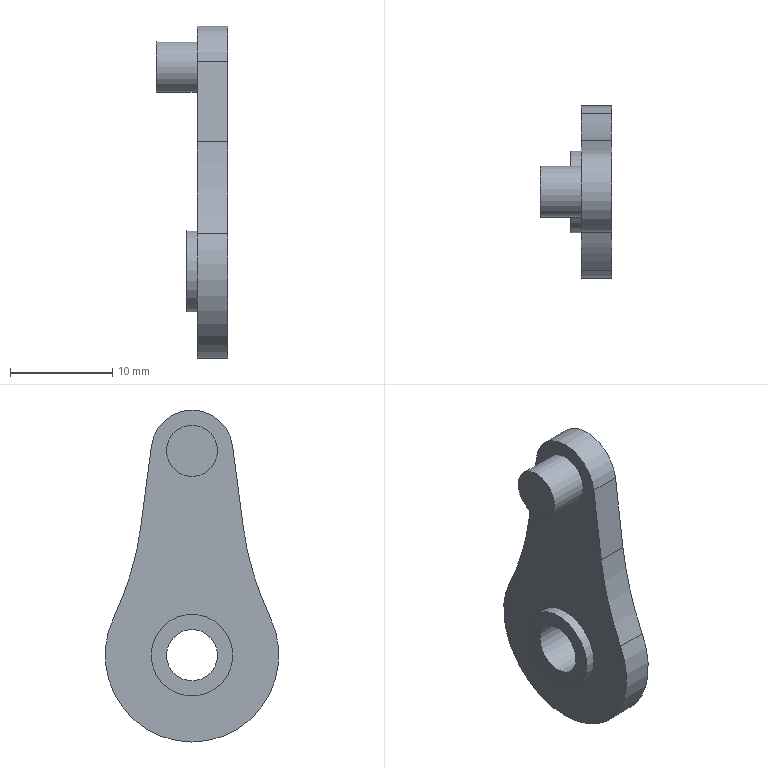Part | STEP file | COMPOUND | 2 solids | 15 faces | box 7 x 17 x 32.5 mm | volume 1174 mm3 | cylinder 8 | plane 7 | commonest cylinder face diameters 8 x3 5 x2 60 x2 17 x1
STEP:
#1=CARTESIAN_POINT('',(0.,0.,0.));
#2=DIRECTION('',(0.,0.,1.));
#3=DIRECTION('',(1.,0.,0.));
#4=AXIS2_PLACEMENT_3D('',#1,#2,#3);
#5=CARTESIAN_POINT('',(3.,4.,-20.));
#6=VERTEX_POINT('',#5);
#7=CARTESIAN_POINT('',(3.,0.,-20.));
#8=DIRECTION('',(1.,0.,0.));
#9=DIRECTION('',(0.,1.,0.));
#10=AXIS2_PLACEMENT_3D('',#7,#8,#9);
#11=CIRCLE('',#10,4.);
#12=CARTESIAN_POINT('',(3.,-1.072,-20.));
#13=DIRECTION('',(1.,0.,0.));
#14=DIRECTION('',(0.,1.,0.));
#15=AXIS2_PLACEMENT_3D('',#12,#13,#14);
#16=PLANE('',#15);
#17=CARTESIAN_POINT('',(1.072,0.));
#18=DIRECTION('',(1.,0.));
#19=AXIS2_PLACEMENT_2D('',#17,#18);
#20=CIRCLE('',#19,4.);
#21=(GEOMETRIC_REPRESENTATION_CONTEXT(2)PARAMETRIC_REPRESENTATION_CONTEXT()REPRESENTATION_CONTEXT('',''));
#22=DEFINITIONAL_REPRESENTATION('',(#20),#21);
#23=PCURVE('',#16,#22);
#24=CARTESIAN_POINT('',(3.,0.,-20.));
#25=DIRECTION('',(-1.,0.,0.));
#26=DIRECTION('',(0.,1.,0.));
#27=AXIS2_PLACEMENT_3D('',#24,#25,#26);
#28=CYLINDRICAL_SURFACE('',#27,4.);
#29=CARTESIAN_POINT('',(6.283,0.));
#30=DIRECTION('',(-1.,0.));
#31=VECTOR('',#30,1.);
#32=LINE('',#29,#31);
#33=(GEOMETRIC_REPRESENTATION_CONTEXT(2)PARAMETRIC_REPRESENTATION_CONTEXT()REPRESENTATION_CONTEXT('',''));
#34=DEFINITIONAL_REPRESENTATION('',(#32),#33);
#35=PCURVE('',#28,#34);
#36=SURFACE_CURVE('',#11,(#23,#35),.PCURVE_S1.);
#37=EDGE_CURVE('',#6,#6,#36,.T.);
#38=ORIENTED_EDGE('',*,*,#37,.T.);
#39=EDGE_LOOP('',(#38));
#40=FACE_BOUND('',#39,.T.);
#41=CARTESIAN_POINT('',(3.,2.5,-20.));
#42=VERTEX_POINT('',#41);
#43=CARTESIAN_POINT('',(3.,0.,-20.));
#44=DIRECTION('',(-1.,0.,0.));
#45=DIRECTION('',(0.,1.,0.));
#46=AXIS2_PLACEMENT_3D('',#43,#44,#45);
#47=CIRCLE('',#46,2.5);
#48=CARTESIAN_POINT('',(3.572,0.));
#49=CARTESIAN_POINT('',(3.572,-4.33));
#50=CARTESIAN_POINT('',(-0.1782,-2.165));
#51=CARTESIAN_POINT('',(-3.928,0.));
#52=CARTESIAN_POINT('',(-0.1782,2.165));
#53=CARTESIAN_POINT('',(3.572,4.33));
#54=CARTESIAN_POINT('',(3.572,0.));
#55=(BOUNDED_CURVE()B_SPLINE_CURVE(2,(#48,#49,#50,#51,#52,#53,#54),.UNSPECIFIED.,.T.,.F.)B_SPLINE_CURVE_WITH_KNOTS((1,2,2,2,2,1),(-2.094,0.,2.094,4.189,6.283,8.378),.UNSPECIFIED.)CURVE()GEOMETRIC_REPRESENTATION_ITEM()RATIONAL_B_SPLINE_CURVE((1.,0.5,1.,0.5,1.,0.5,1.))REPRESENTATION_ITEM(''));
#56=(GEOMETRIC_REPRESENTATION_CONTEXT(2)PARAMETRIC_REPRESENTATION_CONTEXT()REPRESENTATION_CONTEXT('',''));
#57=DEFINITIONAL_REPRESENTATION('',(#55),#56);
#58=PCURVE('',#16,#57);
#59=CARTESIAN_POINT('',(3.,0.,-20.));
#60=DIRECTION('',(-1.,0.,0.));
#61=DIRECTION('',(0.,1.,0.));
#62=AXIS2_PLACEMENT_3D('',#59,#60,#61);
#63=CYLINDRICAL_SURFACE('',#62,2.5);
#64=CARTESIAN_POINT('',(0.,0.));
#65=DIRECTION('',(1.,0.));
#66=VECTOR('',#65,1.);
#67=LINE('',#64,#66);
#68=(GEOMETRIC_REPRESENTATION_CONTEXT(2)PARAMETRIC_REPRESENTATION_CONTEXT()REPRESENTATION_CONTEXT('',''));
#69=DEFINITIONAL_REPRESENTATION('',(#67),#68);
#70=PCURVE('',#63,#69);
#71=SURFACE_CURVE('',#47,(#58,#70),.PCURVE_S1.);
#72=EDGE_CURVE('',#42,#42,#71,.T.);
#73=ORIENTED_EDGE('',*,*,#72,.T.);
#74=EDGE_LOOP('',(#73));
#75=FACE_BOUND('',#74,.T.);
#76=ADVANCED_FACE('',(#40,#75),#16,.T.);
#77=CARTESIAN_POINT('',(-1.,4.,-20.));
#78=VERTEX_POINT('',#77);
#79=CARTESIAN_POINT('',(-1.,0.,-20.));
#80=DIRECTION('',(1.,0.,0.));
#81=DIRECTION('',(0.,1.,0.));
#82=AXIS2_PLACEMENT_3D('',#79,#80,#81);
#83=CIRCLE('',#82,4.);
#84=CARTESIAN_POINT('',(-1.,-1.072,-20.));
#85=DIRECTION('',(1.,0.,0.));
#86=DIRECTION('',(0.,1.,0.));
#87=AXIS2_PLACEMENT_3D('',#84,#85,#86);
#88=PLANE('',#87);
#89=CARTESIAN_POINT('',(1.072,0.));
#90=DIRECTION('',(1.,0.));
#91=AXIS2_PLACEMENT_2D('',#89,#90);
#92=CIRCLE('',#91,4.);
#93=(GEOMETRIC_REPRESENTATION_CONTEXT(2)PARAMETRIC_REPRESENTATION_CONTEXT()REPRESENTATION_CONTEXT('',''));
#94=DEFINITIONAL_REPRESENTATION('',(#92),#93);
#95=PCURVE('',#88,#94);
#96=CARTESIAN_POINT('',(6.283,4.));
#97=DIRECTION('',(-1.,0.));
#98=VECTOR('',#97,1.);
#99=LINE('',#96,#98);
#100=(GEOMETRIC_REPRESENTATION_CONTEXT(2)PARAMETRIC_REPRESENTATION_CONTEXT()REPRESENTATION_CONTEXT('',''));
#101=DEFINITIONAL_REPRESENTATION('',(#99),#100);
#102=PCURVE('',#28,#101);
#103=SURFACE_CURVE('',#83,(#95,#102),.PCURVE_S1.);
#104=EDGE_CURVE('',#78,#78,#103,.T.);
#105=ORIENTED_EDGE('',*,*,#104,.T.);
#106=EDGE_LOOP('',(#105));
#107=FACE_BOUND('',#106,.F.);
#108=CARTESIAN_POINT('',(-1.,2.5,-20.));
#109=VERTEX_POINT('',#108);
#110=CARTESIAN_POINT('',(-1.,0.,-20.));
#111=DIRECTION('',(-1.,0.,0.));
#112=DIRECTION('',(0.,1.,0.));
#113=AXIS2_PLACEMENT_3D('',#110,#111,#112);
#114=CIRCLE('',#113,2.5);
#115=CARTESIAN_POINT('',(3.572,0.));
#116=CARTESIAN_POINT('',(3.572,-4.33));
#117=CARTESIAN_POINT('',(-0.1782,-2.165));
#118=CARTESIAN_POINT('',(-3.928,0.));
#119=CARTESIAN_POINT('',(-0.1782,2.165));
#120=CARTESIAN_POINT('',(3.572,4.33));
#121=CARTESIAN_POINT('',(3.572,0.));
#122=(BOUNDED_CURVE()B_SPLINE_CURVE(2,(#115,#116,#117,#118,#119,#120,#121),.UNSPECIFIED.,.T.,.F.)B_SPLINE_CURVE_WITH_KNOTS((1,2,2,2,2,1),(-2.094,0.,2.094,4.189,6.283,8.378),.UNSPECIFIED.)CURVE()GEOMETRIC_REPRESENTATION_ITEM()RATIONAL_B_SPLINE_CURVE((1.,0.5,1.,0.5,1.,0.5,1.))REPRESENTATION_ITEM(''));
#123=(GEOMETRIC_REPRESENTATION_CONTEXT(2)PARAMETRIC_REPRESENTATION_CONTEXT()REPRESENTATION_CONTEXT('',''));
#124=DEFINITIONAL_REPRESENTATION('',(#122),#123);
#125=PCURVE('',#88,#124);
#126=CARTESIAN_POINT('',(0.,4.));
#127=DIRECTION('',(1.,0.));
#128=VECTOR('',#127,1.);
#129=LINE('',#126,#128);
#130=(GEOMETRIC_REPRESENTATION_CONTEXT(2)PARAMETRIC_REPRESENTATION_CONTEXT()REPRESENTATION_CONTEXT('',''));
#131=DEFINITIONAL_REPRESENTATION('',(#129),#130);
#132=PCURVE('',#63,#131);
#133=SURFACE_CURVE('',#114,(#125,#132),.PCURVE_S1.);
#134=EDGE_CURVE('',#109,#109,#133,.T.);
#135=ORIENTED_EDGE('',*,*,#134,.T.);
#136=EDGE_LOOP('',(#135));
#137=FACE_BOUND('',#136,.F.);
#138=ADVANCED_FACE('',(#107,#137),#88,.F.);
#139=CARTESIAN_POINT('',(3.,4.,-20.));
#140=DIRECTION('',(-1.,0.,0.));
#141=VECTOR('',#140,1.);
#142=LINE('',#139,#141);
#143=CARTESIAN_POINT('',(6.283,0.));
#144=DIRECTION('',(0.,1.));
#145=VECTOR('',#144,1.);
#146=LINE('',#143,#145);
#147=(GEOMETRIC_REPRESENTATION_CONTEXT(2)PARAMETRIC_REPRESENTATION_CONTEXT()REPRESENTATION_CONTEXT('',''));
#148=DEFINITIONAL_REPRESENTATION('',(#146),#147);
#149=PCURVE('',#28,#148);
#150=CARTESIAN_POINT('',(0.,0.));
#151=DIRECTION('',(0.,1.));
#152=VECTOR('',#151,1.);
#153=LINE('',#150,#152);
#154=(GEOMETRIC_REPRESENTATION_CONTEXT(2)PARAMETRIC_REPRESENTATION_CONTEXT()REPRESENTATION_CONTEXT('',''));
#155=DEFINITIONAL_REPRESENTATION('',(#153),#154);
#156=PCURVE('',#28,#155);
#157=SEAM_CURVE('',#142,(#149,#156),.PCURVE_S1.);
#158=EDGE_CURVE('',#6,#78,#157,.T.);
#159=ORIENTED_EDGE('',*,*,#158,.T.);
#160=ORIENTED_EDGE('',*,*,#104,.T.);
#161=ORIENTED_EDGE('',*,*,#158,.F.);
#162=ORIENTED_EDGE('',*,*,#37,.F.);
#163=EDGE_LOOP('',(#159,#160,#161,#162));
#164=FACE_BOUND('',#163,.T.);
#165=ADVANCED_FACE('',(#164),#28,.T.);
#166=ORIENTED_EDGE('',*,*,#72,.T.);
#167=CARTESIAN_POINT('',(3.,2.5,-20.));
#168=DIRECTION('',(-1.,0.,0.));
#169=VECTOR('',#168,1.);
#170=LINE('',#167,#169);
#171=CARTESIAN_POINT('',(6.283,0.));
#172=DIRECTION('',(0.,1.));
#173=VECTOR('',#172,1.);
#174=LINE('',#171,#173);
#175=(GEOMETRIC_REPRESENTATION_CONTEXT(2)PARAMETRIC_REPRESENTATION_CONTEXT()REPRESENTATION_CONTEXT('',''));
#176=DEFINITIONAL_REPRESENTATION('',(#174),#175);
#177=PCURVE('',#63,#176);
#178=CARTESIAN_POINT('',(0.,0.));
#179=DIRECTION('',(0.,1.));
#180=VECTOR('',#179,1.);
#181=LINE('',#178,#180);
#182=(GEOMETRIC_REPRESENTATION_CONTEXT(2)PARAMETRIC_REPRESENTATION_CONTEXT()REPRESENTATION_CONTEXT('',''));
#183=DEFINITIONAL_REPRESENTATION('',(#181),#182);
#184=PCURVE('',#63,#183);
#185=SEAM_CURVE('',#170,(#177,#184),.PCURVE_S1.);
#186=EDGE_CURVE('',#42,#109,#185,.T.);
#187=ORIENTED_EDGE('',*,*,#186,.T.);
#188=ORIENTED_EDGE('',*,*,#134,.F.);
#189=ORIENTED_EDGE('',*,*,#186,.F.);
#190=EDGE_LOOP('',(#166,#187,#188,#189));
#191=FACE_BOUND('',#190,.F.);
#192=ADVANCED_FACE('',(#191),#63,.F.);
#193=CLOSED_SHELL('',(#76,#138,#165,#192));
#194=MANIFOLD_SOLID_BREP('',#193);
#195=CARTESIAN_POINT('',(3.,3.966,0.5224));
#196=VERTEX_POINT('',#195);
#197=CARTESIAN_POINT('',(3.,-3.966,0.5224));
#198=VERTEX_POINT('',#197);
#199=CARTESIAN_POINT('',(3.,0.,0.));
#200=DIRECTION('',(1.,0.,0.));
#201=DIRECTION('',(0.,0.9914,0.1306));
#202=AXIS2_PLACEMENT_3D('',#199,#200,#201);
#203=CIRCLE('',#202,4.);
#204=CARTESIAN_POINT('',(3.,2.773,-12.25));
#205=DIRECTION('',(1.,0.,0.));
#206=DIRECTION('',(0.,1.,0.));
#207=AXIS2_PLACEMENT_3D('',#204,#205,#206);
#208=PLANE('',#207);
#209=CARTESIAN_POINT('',(-2.773,12.25));
#210=DIRECTION('',(0.9914,0.1306));
#211=AXIS2_PLACEMENT_2D('',#209,#210);
#212=CIRCLE('',#211,4.);
#213=(GEOMETRIC_REPRESENTATION_CONTEXT(2)PARAMETRIC_REPRESENTATION_CONTEXT()REPRESENTATION_CONTEXT('',''));
#214=DEFINITIONAL_REPRESENTATION('',(#212),#213);
#215=PCURVE('',#208,#214);
#216=CARTESIAN_POINT('',(0.,0.,0.));
#217=DIRECTION('',(1.,0.,0.));
#218=DIRECTION('',(0.,0.9914,0.1306));
#219=AXIS2_PLACEMENT_3D('',#216,#217,#218);
#220=CYLINDRICAL_SURFACE('',#219,4.);
#221=CARTESIAN_POINT('',(0.,3.));
#222=DIRECTION('',(1.,0.));
#223=VECTOR('',#222,1.);
#224=LINE('',#221,#223);
#225=(GEOMETRIC_REPRESENTATION_CONTEXT(2)PARAMETRIC_REPRESENTATION_CONTEXT()REPRESENTATION_CONTEXT('',''));
#226=DEFINITIONAL_REPRESENTATION('',(#224),#225);
#227=PCURVE('',#220,#226);
#228=SURFACE_CURVE('',#203,(#215,#227),.PCURVE_S1.);
#229=EDGE_CURVE('',#196,#198,#228,.T.);
#230=ORIENTED_EDGE('',*,*,#229,.T.);
#231=CARTESIAN_POINT('',(3.,-5.,-7.33));
#232=VERTEX_POINT('',#231);
#233=CARTESIAN_POINT('',(3.,-3.966,0.5224));
#234=DIRECTION('',(0.,-0.1306,-0.9914));
#235=VECTOR('',#234,1.);
#236=LINE('',#233,#235);
#237=CARTESIAN_POINT('',(-6.738,12.772));
#238=DIRECTION('',(-0.1306,-0.9914));
#239=VECTOR('',#238,1.);
#240=LINE('',#237,#239);
#241=(GEOMETRIC_REPRESENTATION_CONTEXT(2)PARAMETRIC_REPRESENTATION_CONTEXT()REPRESENTATION_CONTEXT('',''));
#242=DEFINITIONAL_REPRESENTATION('',(#240),#241);
#243=PCURVE('',#208,#242);
#244=CARTESIAN_POINT('',(1.5,-4.483,-3.404));
#245=DIRECTION('',(0.,-0.9914,0.1306));
#246=DIRECTION('',(0.,-0.1306,-0.9914));
#247=AXIS2_PLACEMENT_3D('',#244,#245,#246);
#248=PLANE('',#247);
#249=CARTESIAN_POINT('',(-3.96,1.5));
#250=DIRECTION('',(1.,0.));
#251=VECTOR('',#250,1.);
#252=LINE('',#249,#251);
#253=(GEOMETRIC_REPRESENTATION_CONTEXT(2)PARAMETRIC_REPRESENTATION_CONTEXT()REPRESENTATION_CONTEXT('',''));
#254=DEFINITIONAL_REPRESENTATION('',(#252),#253);
#255=PCURVE('',#248,#254);
#256=SURFACE_CURVE('',#236,(#243,#255),.PCURVE_S1.);
#257=EDGE_CURVE('',#198,#232,#256,.T.);
#258=ORIENTED_EDGE('',*,*,#257,.T.);
#259=CARTESIAN_POINT('',(3.,-7.671,-16.338));
#260=VERTEX_POINT('',#259);
#261=CARTESIAN_POINT('',(3.,-34.743,-3.412));
#262=DIRECTION('',(-1.,0.,0.));
#263=DIRECTION('',(0.,0.9914,-0.1306));
#264=AXIS2_PLACEMENT_3D('',#261,#262,#263);
#265=CIRCLE('',#264,30.);
#266=CARTESIAN_POINT('',(-7.773,4.92));
#267=CARTESIAN_POINT('',(-14.558,-46.596));
#268=CARTESIAN_POINT('',(-55.78,-14.961));
#269=CARTESIAN_POINT('',(-97.002,16.674));
#270=CARTESIAN_POINT('',(-48.994,36.555));
#271=CARTESIAN_POINT('',(-0.9868,56.437));
#272=CARTESIAN_POINT('',(-7.773,4.92));
#273=(BOUNDED_CURVE()B_SPLINE_CURVE(2,(#266,#267,#268,#269,#270,#271,#272),.UNSPECIFIED.,.T.,.F.)B_SPLINE_CURVE_WITH_KNOTS((1,2,2,2,2,1),(-2.094,0.,2.094,4.189,6.283,8.378),.UNSPECIFIED.)CURVE()GEOMETRIC_REPRESENTATION_ITEM()RATIONAL_B_SPLINE_CURVE((1.,0.5,1.,0.5,1.,0.5,1.))REPRESENTATION_ITEM(''));
#274=(GEOMETRIC_REPRESENTATION_CONTEXT(2)PARAMETRIC_REPRESENTATION_CONTEXT()REPRESENTATION_CONTEXT('',''));
#275=DEFINITIONAL_REPRESENTATION('',(#273),#274);
#276=PCURVE('',#208,#275);
#277=CARTESIAN_POINT('',(0.,-34.743,-3.412));
#278=DIRECTION('',(1.,0.,0.));
#279=DIRECTION('',(0.,0.9914,-0.1306));
#280=AXIS2_PLACEMENT_3D('',#277,#278,#279);
#281=CYLINDRICAL_SURFACE('',#280,30.);
#282=CARTESIAN_POINT('',(6.283,3.));
#283=DIRECTION('',(-1.,0.));
#284=VECTOR('',#283,1.);
#285=LINE('',#282,#284);
#286=(GEOMETRIC_REPRESENTATION_CONTEXT(2)PARAMETRIC_REPRESENTATION_CONTEXT()REPRESENTATION_CONTEXT('',''));
#287=DEFINITIONAL_REPRESENTATION('',(#285),#286);
#288=PCURVE('',#281,#287);
#289=SURFACE_CURVE('',#265,(#276,#288),.PCURVE_S1.);
#290=EDGE_CURVE('',#232,#260,#289,.T.);
#291=ORIENTED_EDGE('',*,*,#290,.T.);
#292=CARTESIAN_POINT('',(3.,7.671,-16.338));
#293=VERTEX_POINT('',#292);
#294=CARTESIAN_POINT('',(3.,0.,-20.));
#295=DIRECTION('',(1.,0.,0.));
#296=DIRECTION('',(0.,-0.9024,0.4309));
#297=AXIS2_PLACEMENT_3D('',#294,#295,#296);
#298=CIRCLE('',#297,8.5);
#299=CARTESIAN_POINT('',(-2.773,-7.75));
#300=DIRECTION('',(-0.9024,0.4309));
#301=AXIS2_PLACEMENT_2D('',#299,#300);
#302=CIRCLE('',#301,8.5);
#303=(GEOMETRIC_REPRESENTATION_CONTEXT(2)PARAMETRIC_REPRESENTATION_CONTEXT()REPRESENTATION_CONTEXT('',''));
#304=DEFINITIONAL_REPRESENTATION('',(#302),#303);
#305=PCURVE('',#208,#304);
#306=CARTESIAN_POINT('',(0.,0.,-20.));
#307=DIRECTION('',(1.,0.,0.));
#308=DIRECTION('',(0.,-0.9024,0.4309));
#309=AXIS2_PLACEMENT_3D('',#306,#307,#308);
#310=CYLINDRICAL_SURFACE('',#309,8.5);
#311=CARTESIAN_POINT('',(0.,3.));
#312=DIRECTION('',(1.,0.));
#313=VECTOR('',#312,1.);
#314=LINE('',#311,#313);
#315=(GEOMETRIC_REPRESENTATION_CONTEXT(2)PARAMETRIC_REPRESENTATION_CONTEXT()REPRESENTATION_CONTEXT('',''));
#316=DEFINITIONAL_REPRESENTATION('',(#314),#315);
#317=PCURVE('',#310,#316);
#318=SURFACE_CURVE('',#298,(#305,#317),.PCURVE_S1.);
#319=EDGE_CURVE('',#260,#293,#318,.T.);
#320=ORIENTED_EDGE('',*,*,#319,.T.);
#321=CARTESIAN_POINT('',(3.,5.,-7.33));
#322=VERTEX_POINT('',#321);
#323=CARTESIAN_POINT('',(3.,34.743,-3.412));
#324=DIRECTION('',(-1.,0.,0.));
#325=DIRECTION('',(0.,-0.9024,-0.4309));
#326=AXIS2_PLACEMENT_3D('',#323,#324,#325);
#327=CIRCLE('',#326,30.);
#328=CARTESIAN_POINT('',(4.898,-4.088));
#329=CARTESIAN_POINT('',(-17.49,42.803));
#330=CARTESIAN_POINT('',(34.313,38.747));
#331=CARTESIAN_POINT('',(86.116,34.69));
#332=CARTESIAN_POINT('',(56.701,-8.144));
#333=CARTESIAN_POINT('',(27.286,-50.979));
#334=CARTESIAN_POINT('',(4.898,-4.088));
#335=(BOUNDED_CURVE()B_SPLINE_CURVE(2,(#328,#329,#330,#331,#332,#333,#334),.UNSPECIFIED.,.T.,.F.)B_SPLINE_CURVE_WITH_KNOTS((1,2,2,2,2,1),(-2.094,0.,2.094,4.189,6.283,8.378),.UNSPECIFIED.)CURVE()GEOMETRIC_REPRESENTATION_ITEM()RATIONAL_B_SPLINE_CURVE((1.,0.5,1.,0.5,1.,0.5,1.))REPRESENTATION_ITEM(''));
#336=(GEOMETRIC_REPRESENTATION_CONTEXT(2)PARAMETRIC_REPRESENTATION_CONTEXT()REPRESENTATION_CONTEXT('',''));
#337=DEFINITIONAL_REPRESENTATION('',(#335),#336);
#338=PCURVE('',#208,#337);
#339=CARTESIAN_POINT('',(0.,34.743,-3.412));
#340=DIRECTION('',(1.,0.,0.));
#341=DIRECTION('',(0.,-0.9024,-0.4309));
#342=AXIS2_PLACEMENT_3D('',#339,#340,#341);
#343=CYLINDRICAL_SURFACE('',#342,30.);
#344=CARTESIAN_POINT('',(6.283,3.));
#345=DIRECTION('',(-1.,0.));
#346=VECTOR('',#345,1.);
#347=LINE('',#344,#346);
#348=(GEOMETRIC_REPRESENTATION_CONTEXT(2)PARAMETRIC_REPRESENTATION_CONTEXT()REPRESENTATION_CONTEXT('',''));
#349=DEFINITIONAL_REPRESENTATION('',(#347),#348);
#350=PCURVE('',#343,#349);
#351=SURFACE_CURVE('',#327,(#338,#350),.PCURVE_S1.);
#352=EDGE_CURVE('',#293,#322,#351,.T.);
#353=ORIENTED_EDGE('',*,*,#352,.T.);
#354=CARTESIAN_POINT('',(3.,5.,-7.33));
#355=DIRECTION('',(0.,-0.1306,0.9914));
#356=VECTOR('',#355,1.);
#357=LINE('',#354,#356);
#358=CARTESIAN_POINT('',(2.227,4.92));
#359=DIRECTION('',(-0.1306,0.9914));
#360=VECTOR('',#359,1.);
#361=LINE('',#358,#360);
#362=(GEOMETRIC_REPRESENTATION_CONTEXT(2)PARAMETRIC_REPRESENTATION_CONTEXT()REPRESENTATION_CONTEXT('',''));
#363=DEFINITIONAL_REPRESENTATION('',(#361),#362);
#364=PCURVE('',#208,#363);
#365=CARTESIAN_POINT('',(1.5,4.483,-3.404));
#366=DIRECTION('',(0.,0.9914,0.1306));
#367=DIRECTION('',(0.,-0.1306,0.9914));
#368=AXIS2_PLACEMENT_3D('',#365,#366,#367);
#369=PLANE('',#368);
#370=CARTESIAN_POINT('',(-3.96,1.5));
#371=DIRECTION('',(1.,0.));
#372=VECTOR('',#371,1.);
#373=LINE('',#370,#372);
#374=(GEOMETRIC_REPRESENTATION_CONTEXT(2)PARAMETRIC_REPRESENTATION_CONTEXT()REPRESENTATION_CONTEXT('',''));
#375=DEFINITIONAL_REPRESENTATION('',(#373),#374);
#376=PCURVE('',#369,#375);
#377=SURFACE_CURVE('',#357,(#364,#376),.PCURVE_S1.);
#378=EDGE_CURVE('',#322,#196,#377,.T.);
#379=ORIENTED_EDGE('',*,*,#378,.T.);
#380=EDGE_LOOP('',(#230,#258,#291,#320,#353,#379));
#381=FACE_BOUND('',#380,.T.);
#382=CARTESIAN_POINT('',(3.,4.,-20.));
#383=VERTEX_POINT('',#382);
#384=CARTESIAN_POINT('',(3.,0.,-20.));
#385=DIRECTION('',(-1.,0.,0.));
#386=DIRECTION('',(0.,1.,0.));
#387=AXIS2_PLACEMENT_3D('',#384,#385,#386);
#388=CIRCLE('',#387,4.);
#389=CARTESIAN_POINT('',(1.227,-7.75));
#390=CARTESIAN_POINT('',(1.227,-14.678));
#391=CARTESIAN_POINT('',(-4.773,-11.214));
#392=CARTESIAN_POINT('',(-10.773,-7.75));
#393=CARTESIAN_POINT('',(-4.773,-4.286));
#394=CARTESIAN_POINT('',(1.227,-0.8218));
#395=CARTESIAN_POINT('',(1.227,-7.75));
#396=(BOUNDED_CURVE()B_SPLINE_CURVE(2,(#389,#390,#391,#392,#393,#394,#395),.UNSPECIFIED.,.T.,.F.)B_SPLINE_CURVE_WITH_KNOTS((1,2,2,2,2,1),(-2.094,0.,2.094,4.189,6.283,8.378),.UNSPECIFIED.)CURVE()GEOMETRIC_REPRESENTATION_ITEM()RATIONAL_B_SPLINE_CURVE((1.,0.5,1.,0.5,1.,0.5,1.))REPRESENTATION_ITEM(''));
#397=(GEOMETRIC_REPRESENTATION_CONTEXT(2)PARAMETRIC_REPRESENTATION_CONTEXT()REPRESENTATION_CONTEXT('',''));
#398=DEFINITIONAL_REPRESENTATION('',(#396),#397);
#399=PCURVE('',#208,#398);
#400=CARTESIAN_POINT('',(0.,0.,-20.));
#401=DIRECTION('',(1.,0.,0.));
#402=DIRECTION('',(0.,1.,0.));
#403=AXIS2_PLACEMENT_3D('',#400,#401,#402);
#404=CYLINDRICAL_SURFACE('',#403,4.);
#405=CARTESIAN_POINT('',(6.283,3.));
#406=DIRECTION('',(-1.,0.));
#407=VECTOR('',#406,1.);
#408=LINE('',#405,#407);
#409=(GEOMETRIC_REPRESENTATION_CONTEXT(2)PARAMETRIC_REPRESENTATION_CONTEXT()REPRESENTATION_CONTEXT('',''));
#410=DEFINITIONAL_REPRESENTATION('',(#408),#409);
#411=PCURVE('',#404,#410);
#412=SURFACE_CURVE('',#388,(#399,#411),.PCURVE_S1.);
#413=EDGE_CURVE('',#383,#383,#412,.T.);
#414=ORIENTED_EDGE('',*,*,#413,.T.);
#415=EDGE_LOOP('',(#414));
#416=FACE_BOUND('',#415,.T.);
#417=ADVANCED_FACE('',(#381,#416),#208,.T.);
#418=CARTESIAN_POINT('',(0.,3.966,0.5224));
#419=VERTEX_POINT('',#418);
#420=CARTESIAN_POINT('',(0.,-3.966,0.5224));
#421=VERTEX_POINT('',#420);
#422=CARTESIAN_POINT('',(0.,0.,0.));
#423=DIRECTION('',(1.,0.,0.));
#424=DIRECTION('',(0.,0.9914,0.1306));
#425=AXIS2_PLACEMENT_3D('',#422,#423,#424);
#426=CIRCLE('',#425,4.);
#427=CARTESIAN_POINT('',(0.,0.));
#428=DIRECTION('',(1.,0.));
#429=VECTOR('',#428,1.);
#430=LINE('',#427,#429);
#431=(GEOMETRIC_REPRESENTATION_CONTEXT(2)PARAMETRIC_REPRESENTATION_CONTEXT()REPRESENTATION_CONTEXT('',''));
#432=DEFINITIONAL_REPRESENTATION('',(#430),#431);
#433=PCURVE('',#220,#432);
#434=CARTESIAN_POINT('',(0.,2.773,-12.25));
#435=DIRECTION('',(1.,0.,0.));
#436=DIRECTION('',(0.,1.,0.));
#437=AXIS2_PLACEMENT_3D('',#434,#435,#436);
#438=PLANE('',#437);
#439=CARTESIAN_POINT('',(-2.773,12.25));
#440=DIRECTION('',(0.9914,0.1306));
#441=AXIS2_PLACEMENT_2D('',#439,#440);
#442=CIRCLE('',#441,4.);
#443=(GEOMETRIC_REPRESENTATION_CONTEXT(2)PARAMETRIC_REPRESENTATION_CONTEXT()REPRESENTATION_CONTEXT('',''));
#444=DEFINITIONAL_REPRESENTATION('',(#442),#443);
#445=PCURVE('',#438,#444);
#446=SURFACE_CURVE('',#426,(#433,#445),.PCURVE_S1.);
#447=EDGE_CURVE('',#419,#421,#446,.T.);
#448=ORIENTED_EDGE('',*,*,#447,.T.);
#449=CARTESIAN_POINT('',(0.,-3.966,0.5224));
#450=DIRECTION('',(1.,0.,0.));
#451=VECTOR('',#450,1.);
#452=LINE('',#449,#451);
#453=CARTESIAN_POINT('',(2.88,0.));
#454=DIRECTION('',(0.,1.));
#455=VECTOR('',#454,1.);
#456=LINE('',#453,#455);
#457=(GEOMETRIC_REPRESENTATION_CONTEXT(2)PARAMETRIC_REPRESENTATION_CONTEXT()REPRESENTATION_CONTEXT('',''));
#458=DEFINITIONAL_REPRESENTATION('',(#456),#457);
#459=PCURVE('',#220,#458);
#460=CARTESIAN_POINT('',(-3.96,-1.5));
#461=DIRECTION('',(0.,1.));
#462=VECTOR('',#461,1.);
#463=LINE('',#460,#462);
#464=(GEOMETRIC_REPRESENTATION_CONTEXT(2)PARAMETRIC_REPRESENTATION_CONTEXT()REPRESENTATION_CONTEXT('',''));
#465=DEFINITIONAL_REPRESENTATION('',(#463),#464);
#466=PCURVE('',#248,#465);
#467=SURFACE_CURVE('',#452,(#459,#466),.PCURVE_S1.);
#468=EDGE_CURVE('',#421,#198,#467,.T.);
#469=ORIENTED_EDGE('',*,*,#468,.T.);
#470=ORIENTED_EDGE('',*,*,#229,.F.);
#471=CARTESIAN_POINT('',(0.,3.966,0.5224));
#472=DIRECTION('',(1.,0.,0.));
#473=VECTOR('',#472,1.);
#474=LINE('',#471,#473);
#475=CARTESIAN_POINT('',(0.,0.));
#476=DIRECTION('',(0.,1.));
#477=VECTOR('',#476,1.);
#478=LINE('',#475,#477);
#479=(GEOMETRIC_REPRESENTATION_CONTEXT(2)PARAMETRIC_REPRESENTATION_CONTEXT()REPRESENTATION_CONTEXT('',''));
#480=DEFINITIONAL_REPRESENTATION('',(#478),#479);
#481=PCURVE('',#220,#480);
#482=CARTESIAN_POINT('',(3.96,-1.5));
#483=DIRECTION('',(0.,1.));
#484=VECTOR('',#483,1.);
#485=LINE('',#482,#484);
#486=(GEOMETRIC_REPRESENTATION_CONTEXT(2)PARAMETRIC_REPRESENTATION_CONTEXT()REPRESENTATION_CONTEXT('',''));
#487=DEFINITIONAL_REPRESENTATION('',(#485),#486);
#488=PCURVE('',#369,#487);
#489=SURFACE_CURVE('',#474,(#481,#488),.PCURVE_S1.);
#490=EDGE_CURVE('',#419,#196,#489,.T.);
#491=ORIENTED_EDGE('',*,*,#490,.F.);
#492=EDGE_LOOP('',(#448,#469,#470,#491));
#493=FACE_BOUND('',#492,.T.);
#494=ADVANCED_FACE('',(#493),#220,.T.);
#495=CARTESIAN_POINT('',(0.,-5.,-7.33));
#496=VERTEX_POINT('',#495);
#497=CARTESIAN_POINT('',(0.,-3.966,0.5224));
#498=DIRECTION('',(0.,-0.1306,-0.9914));
#499=VECTOR('',#498,1.);
#500=LINE('',#497,#499);
#501=CARTESIAN_POINT('',(-3.96,-1.5));
#502=DIRECTION('',(1.,0.));
#503=VECTOR('',#502,1.);
#504=LINE('',#501,#503);
#505=(GEOMETRIC_REPRESENTATION_CONTEXT(2)PARAMETRIC_REPRESENTATION_CONTEXT()REPRESENTATION_CONTEXT('',''));
#506=DEFINITIONAL_REPRESENTATION('',(#504),#505);
#507=PCURVE('',#248,#506);
#508=CARTESIAN_POINT('',(-6.738,12.772));
#509=DIRECTION('',(-0.1306,-0.9914));
#510=VECTOR('',#509,1.);
#511=LINE('',#508,#510);
#512=(GEOMETRIC_REPRESENTATION_CONTEXT(2)PARAMETRIC_REPRESENTATION_CONTEXT()REPRESENTATION_CONTEXT('',''));
#513=DEFINITIONAL_REPRESENTATION('',(#511),#512);
#514=PCURVE('',#438,#513);
#515=SURFACE_CURVE('',#500,(#507,#514),.PCURVE_S1.);
#516=EDGE_CURVE('',#421,#496,#515,.T.);
#517=ORIENTED_EDGE('',*,*,#516,.T.);
#518=CARTESIAN_POINT('',(0.,-5.,-7.33));
#519=DIRECTION('',(1.,0.,0.));
#520=VECTOR('',#519,1.);
#521=LINE('',#518,#520);
#522=CARTESIAN_POINT('',(3.96,-1.5));
#523=DIRECTION('',(0.,1.));
#524=VECTOR('',#523,1.);
#525=LINE('',#522,#524);
#526=(GEOMETRIC_REPRESENTATION_CONTEXT(2)PARAMETRIC_REPRESENTATION_CONTEXT()REPRESENTATION_CONTEXT('',''));
#527=DEFINITIONAL_REPRESENTATION('',(#525),#526);
#528=PCURVE('',#248,#527);
#529=CARTESIAN_POINT('',(6.283,0.));
#530=DIRECTION('',(0.,1.));
#531=VECTOR('',#530,1.);
#532=LINE('',#529,#531);
#533=(GEOMETRIC_REPRESENTATION_CONTEXT(2)PARAMETRIC_REPRESENTATION_CONTEXT()REPRESENTATION_CONTEXT('',''));
#534=DEFINITIONAL_REPRESENTATION('',(#532),#533);
#535=PCURVE('',#281,#534);
#536=SURFACE_CURVE('',#521,(#528,#535),.PCURVE_S1.);
#537=EDGE_CURVE('',#496,#232,#536,.T.);
#538=ORIENTED_EDGE('',*,*,#537,.T.);
#539=ORIENTED_EDGE('',*,*,#257,.F.);
#540=ORIENTED_EDGE('',*,*,#468,.F.);
#541=EDGE_LOOP('',(#517,#538,#539,#540));
#542=FACE_BOUND('',#541,.T.);
#543=ADVANCED_FACE('',(#542),#248,.T.);
#544=ORIENTED_EDGE('',*,*,#537,.T.);
#545=ORIENTED_EDGE('',*,*,#290,.T.);
#546=CARTESIAN_POINT('',(0.,-7.671,-16.338));
#547=VERTEX_POINT('',#546);
#548=CARTESIAN_POINT('',(0.,-7.671,-16.338));
#549=DIRECTION('',(1.,0.,0.));
#550=VECTOR('',#549,1.);
#551=LINE('',#548,#550);
#552=CARTESIAN_POINT('',(5.969,0.));
#553=DIRECTION('',(0.,1.));
#554=VECTOR('',#553,1.);
#555=LINE('',#552,#554);
#556=(GEOMETRIC_REPRESENTATION_CONTEXT(2)PARAMETRIC_REPRESENTATION_CONTEXT()REPRESENTATION_CONTEXT('',''));
#557=DEFINITIONAL_REPRESENTATION('',(#555),#556);
#558=PCURVE('',#281,#557);
#559=CARTESIAN_POINT('',(0.,0.));
#560=DIRECTION('',(0.,1.));
#561=VECTOR('',#560,1.);
#562=LINE('',#559,#561);
#563=(GEOMETRIC_REPRESENTATION_CONTEXT(2)PARAMETRIC_REPRESENTATION_CONTEXT()REPRESENTATION_CONTEXT('',''));
#564=DEFINITIONAL_REPRESENTATION('',(#562),#563);
#565=PCURVE('',#310,#564);
#566=SURFACE_CURVE('',#551,(#558,#565),.PCURVE_S1.);
#567=EDGE_CURVE('',#547,#260,#566,.T.);
#568=ORIENTED_EDGE('',*,*,#567,.F.);
#569=CARTESIAN_POINT('',(0.,-34.743,-3.412));
#570=DIRECTION('',(-1.,0.,0.));
#571=DIRECTION('',(0.,0.9914,-0.1306));
#572=AXIS2_PLACEMENT_3D('',#569,#570,#571);
#573=CIRCLE('',#572,30.);
#574=CARTESIAN_POINT('',(6.283,0.));
#575=DIRECTION('',(-1.,0.));
#576=VECTOR('',#575,1.);
#577=LINE('',#574,#576);
#578=(GEOMETRIC_REPRESENTATION_CONTEXT(2)PARAMETRIC_REPRESENTATION_CONTEXT()REPRESENTATION_CONTEXT('',''));
#579=DEFINITIONAL_REPRESENTATION('',(#577),#578);
#580=PCURVE('',#281,#579);
#581=CARTESIAN_POINT('',(-7.773,4.92));
#582=CARTESIAN_POINT('',(-14.558,-46.596));
#583=CARTESIAN_POINT('',(-55.78,-14.961));
#584=CARTESIAN_POINT('',(-97.002,16.674));
#585=CARTESIAN_POINT('',(-48.994,36.555));
#586=CARTESIAN_POINT('',(-0.9868,56.437));
#587=CARTESIAN_POINT('',(-7.773,4.92));
#588=(BOUNDED_CURVE()B_SPLINE_CURVE(2,(#581,#582,#583,#584,#585,#586,#587),.UNSPECIFIED.,.T.,.F.)B_SPLINE_CURVE_WITH_KNOTS((1,2,2,2,2,1),(-2.094,0.,2.094,4.189,6.283,8.378),.UNSPECIFIED.)CURVE()GEOMETRIC_REPRESENTATION_ITEM()RATIONAL_B_SPLINE_CURVE((1.,0.5,1.,0.5,1.,0.5,1.))REPRESENTATION_ITEM(''));
#589=(GEOMETRIC_REPRESENTATION_CONTEXT(2)PARAMETRIC_REPRESENTATION_CONTEXT()REPRESENTATION_CONTEXT('',''));
#590=DEFINITIONAL_REPRESENTATION('',(#588),#589);
#591=PCURVE('',#438,#590);
#592=SURFACE_CURVE('',#573,(#580,#591),.PCURVE_S1.);
#593=EDGE_CURVE('',#496,#547,#592,.T.);
#594=ORIENTED_EDGE('',*,*,#593,.F.);
#595=EDGE_LOOP('',(#544,#545,#568,#594));
#596=FACE_BOUND('',#595,.F.);
#597=ADVANCED_FACE('',(#596),#281,.F.);
#598=CARTESIAN_POINT('',(0.,7.671,-16.338));
#599=VERTEX_POINT('',#598);
#600=CARTESIAN_POINT('',(0.,0.,-20.));
#601=DIRECTION('',(1.,0.,0.));
#602=DIRECTION('',(0.,-0.9024,0.4309));
#603=AXIS2_PLACEMENT_3D('',#600,#601,#602);
#604=CIRCLE('',#603,8.5);
#605=CARTESIAN_POINT('',(0.,0.));
#606=DIRECTION('',(1.,0.));
#607=VECTOR('',#606,1.);
#608=LINE('',#605,#607);
#609=(GEOMETRIC_REPRESENTATION_CONTEXT(2)PARAMETRIC_REPRESENTATION_CONTEXT()REPRESENTATION_CONTEXT('',''));
#610=DEFINITIONAL_REPRESENTATION('',(#608),#609);
#611=PCURVE('',#310,#610);
#612=CARTESIAN_POINT('',(-2.773,-7.75));
#613=DIRECTION('',(-0.9024,0.4309));
#614=AXIS2_PLACEMENT_2D('',#612,#613);
#615=CIRCLE('',#614,8.5);
#616=(GEOMETRIC_REPRESENTATION_CONTEXT(2)PARAMETRIC_REPRESENTATION_CONTEXT()REPRESENTATION_CONTEXT('',''));
#617=DEFINITIONAL_REPRESENTATION('',(#615),#616);
#618=PCURVE('',#438,#617);
#619=SURFACE_CURVE('',#604,(#611,#618),.PCURVE_S1.);
#620=EDGE_CURVE('',#547,#599,#619,.T.);
#621=ORIENTED_EDGE('',*,*,#620,.T.);
#622=CARTESIAN_POINT('',(0.,7.671,-16.338));
#623=DIRECTION('',(1.,0.,0.));
#624=VECTOR('',#623,1.);
#625=LINE('',#622,#624);
#626=CARTESIAN_POINT('',(4.032,0.));
#627=DIRECTION('',(0.,1.));
#628=VECTOR('',#627,1.);
#629=LINE('',#626,#628);
#630=(GEOMETRIC_REPRESENTATION_CONTEXT(2)PARAMETRIC_REPRESENTATION_CONTEXT()REPRESENTATION_CONTEXT('',''));
#631=DEFINITIONAL_REPRESENTATION('',(#629),#630);
#632=PCURVE('',#310,#631);
#633=CARTESIAN_POINT('',(6.283,0.));
#634=DIRECTION('',(0.,1.));
#635=VECTOR('',#634,1.);
#636=LINE('',#633,#635);
#637=(GEOMETRIC_REPRESENTATION_CONTEXT(2)PARAMETRIC_REPRESENTATION_CONTEXT()REPRESENTATION_CONTEXT('',''));
#638=DEFINITIONAL_REPRESENTATION('',(#636),#637);
#639=PCURVE('',#343,#638);
#640=SURFACE_CURVE('',#625,(#632,#639),.PCURVE_S1.);
#641=EDGE_CURVE('',#599,#293,#640,.T.);
#642=ORIENTED_EDGE('',*,*,#641,.T.);
#643=ORIENTED_EDGE('',*,*,#319,.F.);
#644=ORIENTED_EDGE('',*,*,#567,.F.);
#645=EDGE_LOOP('',(#621,#642,#643,#644));
#646=FACE_BOUND('',#645,.T.);
#647=ADVANCED_FACE('',(#646),#310,.T.);
#648=ORIENTED_EDGE('',*,*,#641,.T.);
#649=ORIENTED_EDGE('',*,*,#352,.T.);
#650=CARTESIAN_POINT('',(0.,5.,-7.33));
#651=VERTEX_POINT('',#650);
#652=CARTESIAN_POINT('',(0.,5.,-7.33));
#653=DIRECTION('',(1.,0.,0.));
#654=VECTOR('',#653,1.);
#655=LINE('',#652,#654);
#656=CARTESIAN_POINT('',(5.969,0.));
#657=DIRECTION('',(0.,1.));
#658=VECTOR('',#657,1.);
#659=LINE('',#656,#658);
#660=(GEOMETRIC_REPRESENTATION_CONTEXT(2)PARAMETRIC_REPRESENTATION_CONTEXT()REPRESENTATION_CONTEXT('',''));
#661=DEFINITIONAL_REPRESENTATION('',(#659),#660);
#662=PCURVE('',#343,#661);
#663=CARTESIAN_POINT('',(-3.96,-1.5));
#664=DIRECTION('',(0.,1.));
#665=VECTOR('',#664,1.);
#666=LINE('',#663,#665);
#667=(GEOMETRIC_REPRESENTATION_CONTEXT(2)PARAMETRIC_REPRESENTATION_CONTEXT()REPRESENTATION_CONTEXT('',''));
#668=DEFINITIONAL_REPRESENTATION('',(#666),#667);
#669=PCURVE('',#369,#668);
#670=SURFACE_CURVE('',#655,(#662,#669),.PCURVE_S1.);
#671=EDGE_CURVE('',#651,#322,#670,.T.);
#672=ORIENTED_EDGE('',*,*,#671,.F.);
#673=CARTESIAN_POINT('',(0.,34.743,-3.412));
#674=DIRECTION('',(-1.,0.,0.));
#675=DIRECTION('',(0.,-0.9024,-0.4309));
#676=AXIS2_PLACEMENT_3D('',#673,#674,#675);
#677=CIRCLE('',#676,30.);
#678=CARTESIAN_POINT('',(6.283,0.));
#679=DIRECTION('',(-1.,0.));
#680=VECTOR('',#679,1.);
#681=LINE('',#678,#680);
#682=(GEOMETRIC_REPRESENTATION_CONTEXT(2)PARAMETRIC_REPRESENTATION_CONTEXT()REPRESENTATION_CONTEXT('',''));
#683=DEFINITIONAL_REPRESENTATION('',(#681),#682);
#684=PCURVE('',#343,#683);
#685=CARTESIAN_POINT('',(4.898,-4.088));
#686=CARTESIAN_POINT('',(-17.49,42.803));
#687=CARTESIAN_POINT('',(34.313,38.747));
#688=CARTESIAN_POINT('',(86.116,34.69));
#689=CARTESIAN_POINT('',(56.701,-8.144));
#690=CARTESIAN_POINT('',(27.286,-50.979));
#691=CARTESIAN_POINT('',(4.898,-4.088));
#692=(BOUNDED_CURVE()B_SPLINE_CURVE(2,(#685,#686,#687,#688,#689,#690,#691),.UNSPECIFIED.,.T.,.F.)B_SPLINE_CURVE_WITH_KNOTS((1,2,2,2,2,1),(-2.094,0.,2.094,4.189,6.283,8.378),.UNSPECIFIED.)CURVE()GEOMETRIC_REPRESENTATION_ITEM()RATIONAL_B_SPLINE_CURVE((1.,0.5,1.,0.5,1.,0.5,1.))REPRESENTATION_ITEM(''));
#693=(GEOMETRIC_REPRESENTATION_CONTEXT(2)PARAMETRIC_REPRESENTATION_CONTEXT()REPRESENTATION_CONTEXT('',''));
#694=DEFINITIONAL_REPRESENTATION('',(#692),#693);
#695=PCURVE('',#438,#694);
#696=SURFACE_CURVE('',#677,(#684,#695),.PCURVE_S1.);
#697=EDGE_CURVE('',#599,#651,#696,.T.);
#698=ORIENTED_EDGE('',*,*,#697,.F.);
#699=EDGE_LOOP('',(#648,#649,#672,#698));
#700=FACE_BOUND('',#699,.F.);
#701=ADVANCED_FACE('',(#700),#343,.F.);
#702=CARTESIAN_POINT('',(0.,5.,-7.33));
#703=DIRECTION('',(0.,-0.1306,0.9914));
#704=VECTOR('',#703,1.);
#705=LINE('',#702,#704);
#706=CARTESIAN_POINT('',(-3.96,-1.5));
#707=DIRECTION('',(1.,0.));
#708=VECTOR('',#707,1.);
#709=LINE('',#706,#708);
#710=(GEOMETRIC_REPRESENTATION_CONTEXT(2)PARAMETRIC_REPRESENTATION_CONTEXT()REPRESENTATION_CONTEXT('',''));
#711=DEFINITIONAL_REPRESENTATION('',(#709),#710);
#712=PCURVE('',#369,#711);
#713=CARTESIAN_POINT('',(2.227,4.92));
#714=DIRECTION('',(-0.1306,0.9914));
#715=VECTOR('',#714,1.);
#716=LINE('',#713,#715);
#717=(GEOMETRIC_REPRESENTATION_CONTEXT(2)PARAMETRIC_REPRESENTATION_CONTEXT()REPRESENTATION_CONTEXT('',''));
#718=DEFINITIONAL_REPRESENTATION('',(#716),#717);
#719=PCURVE('',#438,#718);
#720=SURFACE_CURVE('',#705,(#712,#719),.PCURVE_S1.);
#721=EDGE_CURVE('',#651,#419,#720,.T.);
#722=ORIENTED_EDGE('',*,*,#721,.T.);
#723=ORIENTED_EDGE('',*,*,#490,.T.);
#724=ORIENTED_EDGE('',*,*,#378,.F.);
#725=ORIENTED_EDGE('',*,*,#671,.F.);
#726=EDGE_LOOP('',(#722,#723,#724,#725));
#727=FACE_BOUND('',#726,.T.);
#728=ADVANCED_FACE('',(#727),#369,.T.);
#729=CARTESIAN_POINT('',(0.,4.,-20.));
#730=VERTEX_POINT('',#729);
#731=CARTESIAN_POINT('',(0.,4.,-20.));
#732=DIRECTION('',(1.,0.,0.));
#733=VECTOR('',#732,1.);
#734=LINE('',#731,#733);
#735=CARTESIAN_POINT('',(6.283,0.));
#736=DIRECTION('',(0.,1.));
#737=VECTOR('',#736,1.);
#738=LINE('',#735,#737);
#739=(GEOMETRIC_REPRESENTATION_CONTEXT(2)PARAMETRIC_REPRESENTATION_CONTEXT()REPRESENTATION_CONTEXT('',''));
#740=DEFINITIONAL_REPRESENTATION('',(#738),#739);
#741=PCURVE('',#404,#740);
#742=CARTESIAN_POINT('',(0.,0.));
#743=DIRECTION('',(0.,1.));
#744=VECTOR('',#743,1.);
#745=LINE('',#742,#744);
#746=(GEOMETRIC_REPRESENTATION_CONTEXT(2)PARAMETRIC_REPRESENTATION_CONTEXT()REPRESENTATION_CONTEXT('',''));
#747=DEFINITIONAL_REPRESENTATION('',(#745),#746);
#748=PCURVE('',#404,#747);
#749=SEAM_CURVE('',#734,(#741,#748),.PCURVE_S1.);
#750=EDGE_CURVE('',#730,#383,#749,.T.);
#751=ORIENTED_EDGE('',*,*,#750,.T.);
#752=ORIENTED_EDGE('',*,*,#413,.T.);
#753=ORIENTED_EDGE('',*,*,#750,.F.);
#754=CARTESIAN_POINT('',(0.,0.,-20.));
#755=DIRECTION('',(-1.,0.,0.));
#756=DIRECTION('',(0.,1.,0.));
#757=AXIS2_PLACEMENT_3D('',#754,#755,#756);
#758=CIRCLE('',#757,4.);
#759=CARTESIAN_POINT('',(6.283,0.));
#760=DIRECTION('',(-1.,0.));
#761=VECTOR('',#760,1.);
#762=LINE('',#759,#761);
#763=(GEOMETRIC_REPRESENTATION_CONTEXT(2)PARAMETRIC_REPRESENTATION_CONTEXT()REPRESENTATION_CONTEXT('',''));
#764=DEFINITIONAL_REPRESENTATION('',(#762),#763);
#765=PCURVE('',#404,#764);
#766=CARTESIAN_POINT('',(1.227,-7.75));
#767=CARTESIAN_POINT('',(1.227,-14.678));
#768=CARTESIAN_POINT('',(-4.773,-11.214));
#769=CARTESIAN_POINT('',(-10.773,-7.75));
#770=CARTESIAN_POINT('',(-4.773,-4.286));
#771=CARTESIAN_POINT('',(1.227,-0.8218));
#772=CARTESIAN_POINT('',(1.227,-7.75));
#773=(BOUNDED_CURVE()B_SPLINE_CURVE(2,(#766,#767,#768,#769,#770,#771,#772),.UNSPECIFIED.,.T.,.F.)B_SPLINE_CURVE_WITH_KNOTS((1,2,2,2,2,1),(-2.094,0.,2.094,4.189,6.283,8.378),.UNSPECIFIED.)CURVE()GEOMETRIC_REPRESENTATION_ITEM()RATIONAL_B_SPLINE_CURVE((1.,0.5,1.,0.5,1.,0.5,1.))REPRESENTATION_ITEM(''));
#774=(GEOMETRIC_REPRESENTATION_CONTEXT(2)PARAMETRIC_REPRESENTATION_CONTEXT()REPRESENTATION_CONTEXT('',''));
#775=DEFINITIONAL_REPRESENTATION('',(#773),#774);
#776=PCURVE('',#438,#775);
#777=SURFACE_CURVE('',#758,(#765,#776),.PCURVE_S1.);
#778=EDGE_CURVE('',#730,#730,#777,.T.);
#779=ORIENTED_EDGE('',*,*,#778,.F.);
#780=EDGE_LOOP('',(#751,#752,#753,#779));
#781=FACE_BOUND('',#780,.F.);
#782=ADVANCED_FACE('',(#781),#404,.F.);
#783=ORIENTED_EDGE('',*,*,#447,.T.);
#784=ORIENTED_EDGE('',*,*,#516,.T.);
#785=ORIENTED_EDGE('',*,*,#593,.T.);
#786=ORIENTED_EDGE('',*,*,#620,.T.);
#787=ORIENTED_EDGE('',*,*,#697,.T.);
#788=ORIENTED_EDGE('',*,*,#721,.T.);
#789=EDGE_LOOP('',(#783,#784,#785,#786,#787,#788));
#790=FACE_BOUND('',#789,.F.);
#791=CARTESIAN_POINT('',(0.,-2.5,0.));
#792=VERTEX_POINT('',#791);
#793=CARTESIAN_POINT('',(0.,0.,0.));
#794=DIRECTION('',(-1.,0.,0.));
#795=DIRECTION('',(0.,-1.,0.));
#796=AXIS2_PLACEMENT_3D('',#793,#794,#795);
#797=CIRCLE('',#796,2.5);
#798=CARTESIAN_POINT('',(-5.273,12.25));
#799=CARTESIAN_POINT('',(-5.273,16.58));
#800=CARTESIAN_POINT('',(-1.523,14.415));
#801=CARTESIAN_POINT('',(2.227,12.25));
#802=CARTESIAN_POINT('',(-1.523,10.085));
#803=CARTESIAN_POINT('',(-5.273,7.92));
#804=CARTESIAN_POINT('',(-5.273,12.25));
#805=(BOUNDED_CURVE()B_SPLINE_CURVE(2,(#798,#799,#800,#801,#802,#803,#804),.UNSPECIFIED.,.T.,.F.)B_SPLINE_CURVE_WITH_KNOTS((1,2,2,2,2,1),(-2.094,0.,2.094,4.189,6.283,8.378),.UNSPECIFIED.)CURVE()GEOMETRIC_REPRESENTATION_ITEM()RATIONAL_B_SPLINE_CURVE((1.,0.5,1.,0.5,1.,0.5,1.))REPRESENTATION_ITEM(''));
#806=(GEOMETRIC_REPRESENTATION_CONTEXT(2)PARAMETRIC_REPRESENTATION_CONTEXT()REPRESENTATION_CONTEXT('',''));
#807=DEFINITIONAL_REPRESENTATION('',(#805),#806);
#808=PCURVE('',#438,#807);
#809=CARTESIAN_POINT('',(0.,0.,0.));
#810=DIRECTION('',(-1.,0.,0.));
#811=DIRECTION('',(0.,-1.,0.));
#812=AXIS2_PLACEMENT_3D('',#809,#810,#811);
#813=CYLINDRICAL_SURFACE('',#812,2.5);
#814=CARTESIAN_POINT('',(0.,0.));
#815=DIRECTION('',(1.,0.));
#816=VECTOR('',#815,1.);
#817=LINE('',#814,#816);
#818=(GEOMETRIC_REPRESENTATION_CONTEXT(2)PARAMETRIC_REPRESENTATION_CONTEXT()REPRESENTATION_CONTEXT('',''));
#819=DEFINITIONAL_REPRESENTATION('',(#817),#818);
#820=PCURVE('',#813,#819);
#821=SURFACE_CURVE('',#797,(#808,#820),.PCURVE_S1.);
#822=EDGE_CURVE('',#792,#792,#821,.T.);
#823=ORIENTED_EDGE('',*,*,#822,.T.);
#824=EDGE_LOOP('',(#823));
#825=FACE_BOUND('',#824,.F.);
#826=ORIENTED_EDGE('',*,*,#778,.T.);
#827=EDGE_LOOP('',(#826));
#828=FACE_BOUND('',#827,.F.);
#829=ADVANCED_FACE('',(#790,#825,#828),#438,.F.);
#830=ORIENTED_EDGE('',*,*,#822,.T.);
#831=CARTESIAN_POINT('',(-4.,-2.5,0.));
#832=VERTEX_POINT('',#831);
#833=CARTESIAN_POINT('',(0.,-2.5,0.));
#834=DIRECTION('',(-1.,0.,0.));
#835=VECTOR('',#834,1.);
#836=LINE('',#833,#835);
#837=CARTESIAN_POINT('',(6.283,0.));
#838=DIRECTION('',(0.,1.));
#839=VECTOR('',#838,1.);
#840=LINE('',#837,#839);
#841=(GEOMETRIC_REPRESENTATION_CONTEXT(2)PARAMETRIC_REPRESENTATION_CONTEXT()REPRESENTATION_CONTEXT('',''));
#842=DEFINITIONAL_REPRESENTATION('',(#840),#841);
#843=PCURVE('',#813,#842);
#844=CARTESIAN_POINT('',(0.,0.));
#845=DIRECTION('',(0.,1.));
#846=VECTOR('',#845,1.);
#847=LINE('',#844,#846);
#848=(GEOMETRIC_REPRESENTATION_CONTEXT(2)PARAMETRIC_REPRESENTATION_CONTEXT()REPRESENTATION_CONTEXT('',''));
#849=DEFINITIONAL_REPRESENTATION('',(#847),#848);
#850=PCURVE('',#813,#849);
#851=SEAM_CURVE('',#836,(#843,#850),.PCURVE_S1.);
#852=EDGE_CURVE('',#792,#832,#851,.T.);
#853=ORIENTED_EDGE('',*,*,#852,.T.);
#854=CARTESIAN_POINT('',(-4.,0.,0.));
#855=DIRECTION('',(-1.,0.,0.));
#856=DIRECTION('',(0.,-1.,0.));
#857=AXIS2_PLACEMENT_3D('',#854,#855,#856);
#858=CIRCLE('',#857,2.5);
#859=CARTESIAN_POINT('',(0.,4.));
#860=DIRECTION('',(1.,0.));
#861=VECTOR('',#860,1.);
#862=LINE('',#859,#861);
#863=(GEOMETRIC_REPRESENTATION_CONTEXT(2)PARAMETRIC_REPRESENTATION_CONTEXT()REPRESENTATION_CONTEXT('',''));
#864=DEFINITIONAL_REPRESENTATION('',(#862),#863);
#865=PCURVE('',#813,#864);
#866=CARTESIAN_POINT('',(-4.,0.6699,0.));
#867=DIRECTION('',(-1.,0.,0.));
#868=DIRECTION('',(0.,-1.,0.));
#869=AXIS2_PLACEMENT_3D('',#866,#867,#868);
#870=PLANE('',#869);
#871=CARTESIAN_POINT('',(0.6699,0.));
#872=DIRECTION('',(1.,0.));
#873=AXIS2_PLACEMENT_2D('',#871,#872);
#874=CIRCLE('',#873,2.5);
#875=(GEOMETRIC_REPRESENTATION_CONTEXT(2)PARAMETRIC_REPRESENTATION_CONTEXT()REPRESENTATION_CONTEXT('',''));
#876=DEFINITIONAL_REPRESENTATION('',(#874),#875);
#877=PCURVE('',#870,#876);
#878=SURFACE_CURVE('',#858,(#865,#877),.PCURVE_S1.);
#879=EDGE_CURVE('',#832,#832,#878,.T.);
#880=ORIENTED_EDGE('',*,*,#879,.F.);
#881=ORIENTED_EDGE('',*,*,#852,.F.);
#882=EDGE_LOOP('',(#830,#853,#880,#881));
#883=FACE_BOUND('',#882,.T.);
#884=ADVANCED_FACE('',(#883),#813,.T.);
#885=ORIENTED_EDGE('',*,*,#879,.T.);
#886=EDGE_LOOP('',(#885));
#887=FACE_BOUND('',#886,.T.);
#888=ADVANCED_FACE('',(#887),#870,.T.);
#889=CLOSED_SHELL('',(#417,#494,#543,#597,#647,#701,#728,#782,#829,#884,#888));
#890=MANIFOLD_SOLID_BREP('',#889);
#891=(LENGTH_UNIT()NAMED_UNIT(*)SI_UNIT(.MILLI.,.METRE.));
#892=UNCERTAINTY_MEASURE_WITH_UNIT(LENGTH_MEASURE(0.0000001),#891,'','');
#893=(NAMED_UNIT(*)PLANE_ANGLE_UNIT()SI_UNIT($,.RADIAN.));
#894=(NAMED_UNIT(*)SI_UNIT($,.STERADIAN.)SOLID_ANGLE_UNIT());
#895=(GEOMETRIC_REPRESENTATION_CONTEXT(3)GLOBAL_UNCERTAINTY_ASSIGNED_CONTEXT((#892))GLOBAL_UNIT_ASSIGNED_CONTEXT((#891,#893,#894))REPRESENTATION_CONTEXT('',''));
#896=SHAPE_REPRESENTATION('',(#4,#194,#890),#895);